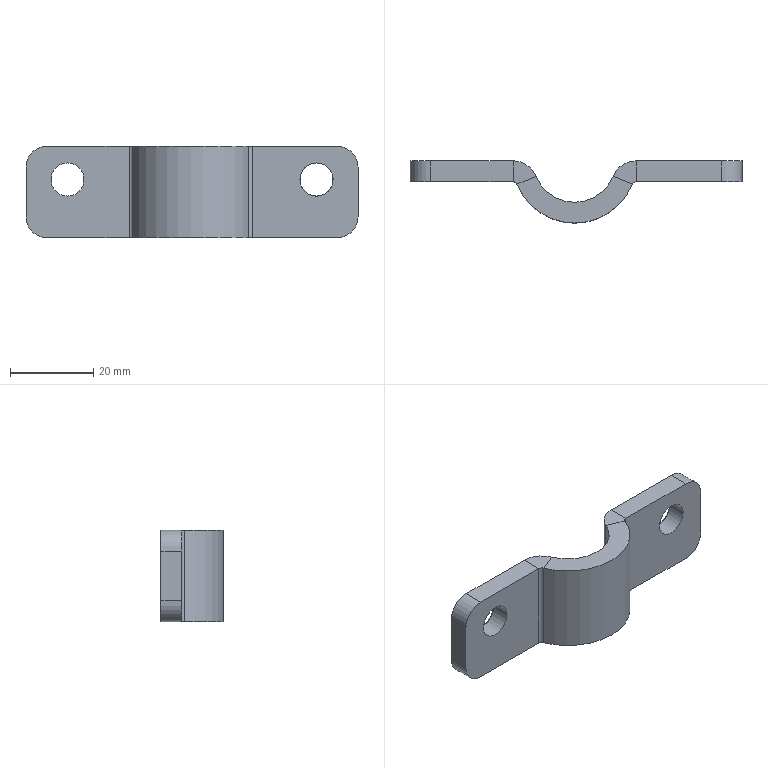Part | STEP file | 6100106 | 1 solid | 30 faces | box 80 x 15 x 22 mm | volume 9096 mm3 | plane 16 | cylinder 12 | cone 2 | commonest cylinder face diameters 10 x4 2 x2 8 x2 12 x2 20 x1 30 x1